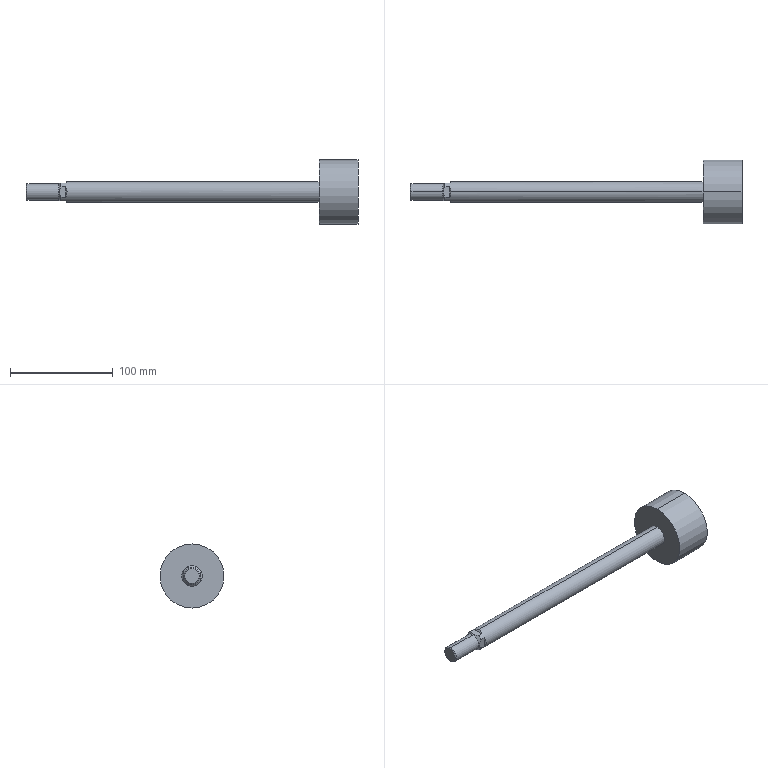Part | SolidWorks | features BaseBody 1 | 1 solid | 21 faces | box 323.5 x 62.5 x 62.5 mm | volume 202274 mm3 | plane 11 | cylinder 6 | cone 4 | commonest cylinder face diameters 16 x2 20 x2 62.5 x2
STEP:
#1=CARTESIAN_POINT('',(216.5,0.,10.));
#2=VERTEX_POINT('',#1);
#3=CARTESIAN_POINT('',(216.5,0.,-10.));
#4=VERTEX_POINT('',#3);
#5=CARTESIAN_POINT('',(216.5,0.,0.));
#6=DIRECTION('',(-1.,0.,0.));
#7=DIRECTION('',(0.,0.,1.));
#8=AXIS2_PLACEMENT_3D('',#5,#6,#7);
#9=CIRCLE('',#8,10.);
#10=EDGE_CURVE('',#2,#4,#9,.T.);
#11=ORIENTED_EDGE('',*,*,#10,.T.);
#12=CARTESIAN_POINT('',(-29.,0.,-10.));
#13=VERTEX_POINT('',#12);
#14=CARTESIAN_POINT('',(254.5,0.,-10.));
#15=DIRECTION('',(-1.,0.,0.));
#16=VECTOR('',#15,1000.);
#17=LINE('',#14,#16);
#18=EDGE_CURVE('',#4,#13,#17,.T.);
#19=ORIENTED_EDGE('',*,*,#18,.T.);
#20=CARTESIAN_POINT('',(-30.5,5.268,-8.5));
#21=VERTEX_POINT('',#20);
#22=CARTESIAN_POINT('',(-29.,0.,-10.));
#23=CARTESIAN_POINT('',(-29.,1.873,-10.));
#24=CARTESIAN_POINT('',(-29.513,3.675,-9.487));
#25=CARTESIAN_POINT('',(-30.5,5.268,-8.5));
#26=(BOUNDED_CURVE()B_SPLINE_CURVE(3,(#22,#23,#24,#25),.UNSPECIFIED.,.F.,.T.)B_SPLINE_CURVE_WITH_KNOTS((4,4),(3.142,3.696),.UNSPECIFIED.)CURVE()GEOMETRIC_REPRESENTATION_ITEM()RATIONAL_B_SPLINE_CURVE((1.,0.9745,0.9745,1.))REPRESENTATION_ITEM(''));
#27=EDGE_CURVE('',#13,#21,#26,.T.);
#28=ORIENTED_EDGE('',*,*,#27,.T.);
#29=CARTESIAN_POINT('',(-35.,5.268,-8.5));
#30=VERTEX_POINT('',#29);
#31=CARTESIAN_POINT('',(254.5,5.268,-8.5));
#32=DIRECTION('',(-1.,0.,0.));
#33=VECTOR('',#32,1000.);
#34=LINE('',#31,#33);
#35=EDGE_CURVE('',#21,#30,#34,.T.);
#36=ORIENTED_EDGE('',*,*,#35,.T.);
#37=CARTESIAN_POINT('',(-35.,8.5,-5.268));
#38=VERTEX_POINT('',#37);
#39=CARTESIAN_POINT('',(-35.,0.,0.));
#40=DIRECTION('',(1.,0.,0.));
#41=DIRECTION('',(0.,0.,1.));
#42=AXIS2_PLACEMENT_3D('',#39,#40,#41);
#43=CIRCLE('',#42,10.);
#44=EDGE_CURVE('',#30,#38,#43,.T.);
#45=ORIENTED_EDGE('',*,*,#44,.T.);
#46=CARTESIAN_POINT('',(-30.5,8.5,-5.268));
#47=VERTEX_POINT('',#46);
#48=CARTESIAN_POINT('',(254.5,8.5,-5.268));
#49=DIRECTION('',(1.,0.,0.));
#50=VECTOR('',#49,1000.);
#51=LINE('',#48,#50);
#52=EDGE_CURVE('',#38,#47,#51,.T.);
#53=ORIENTED_EDGE('',*,*,#52,.T.);
#54=CARTESIAN_POINT('',(-30.5,8.5,5.268));
#55=VERTEX_POINT('',#54);
#56=CARTESIAN_POINT('',(-30.5,8.5,-5.268));
#57=CARTESIAN_POINT('',(-28.444,10.556,-1.951));
#58=CARTESIAN_POINT('',(-28.444,10.556,1.951));
#59=CARTESIAN_POINT('',(-30.5,8.5,5.268));
#60=(BOUNDED_CURVE()B_SPLINE_CURVE(3,(#56,#57,#58,#59),.UNSPECIFIED.,.F.,.T.)B_SPLINE_CURVE_WITH_KNOTS((4,4),(2.587,3.696),.UNSPECIFIED.)CURVE()GEOMETRIC_REPRESENTATION_ITEM()RATIONAL_B_SPLINE_CURVE((1.,0.9,0.9,1.))REPRESENTATION_ITEM(''));
#61=EDGE_CURVE('',#47,#55,#60,.T.);
#62=ORIENTED_EDGE('',*,*,#61,.T.);
#63=CARTESIAN_POINT('',(-35.,8.5,5.268));
#64=VERTEX_POINT('',#63);
#65=CARTESIAN_POINT('',(254.5,8.5,5.268));
#66=DIRECTION('',(-1.,0.,0.));
#67=VECTOR('',#66,1000.);
#68=LINE('',#65,#67);
#69=EDGE_CURVE('',#55,#64,#68,.T.);
#70=ORIENTED_EDGE('',*,*,#69,.T.);
#71=CARTESIAN_POINT('',(-35.,5.268,8.5));
#72=VERTEX_POINT('',#71);
#73=CARTESIAN_POINT('',(-35.,0.,0.));
#74=DIRECTION('',(1.,0.,0.));
#75=DIRECTION('',(0.,0.,1.));
#76=AXIS2_PLACEMENT_3D('',#73,#74,#75);
#77=CIRCLE('',#76,10.);
#78=EDGE_CURVE('',#64,#72,#77,.T.);
#79=ORIENTED_EDGE('',*,*,#78,.T.);
#80=CARTESIAN_POINT('',(-30.5,5.268,8.5));
#81=VERTEX_POINT('',#80);
#82=CARTESIAN_POINT('',(254.5,5.268,8.5));
#83=DIRECTION('',(1.,0.,0.));
#84=VECTOR('',#83,1000.);
#85=LINE('',#82,#84);
#86=EDGE_CURVE('',#72,#81,#85,.T.);
#87=ORIENTED_EDGE('',*,*,#86,.T.);
#88=CARTESIAN_POINT('',(-29.,0.,10.));
#89=VERTEX_POINT('',#88);
#90=CARTESIAN_POINT('',(-30.5,5.268,8.5));
#91=CARTESIAN_POINT('',(-29.513,3.675,9.487));
#92=CARTESIAN_POINT('',(-29.,1.873,10.));
#93=CARTESIAN_POINT('',(-29.,0.,10.));
#94=(BOUNDED_CURVE()B_SPLINE_CURVE(3,(#90,#91,#92,#93),.UNSPECIFIED.,.F.,.F.)B_SPLINE_CURVE_WITH_KNOTS((4,4),(2.587,3.142),.UNSPECIFIED.)CURVE()GEOMETRIC_REPRESENTATION_ITEM()RATIONAL_B_SPLINE_CURVE((1.,0.9745,0.9745,1.))REPRESENTATION_ITEM(''));
#95=EDGE_CURVE('',#81,#89,#94,.T.);
#96=ORIENTED_EDGE('',*,*,#95,.T.);
#97=CARTESIAN_POINT('',(254.5,0.,10.));
#98=DIRECTION('',(-1.,0.,0.));
#99=VECTOR('',#98,1000.);
#100=LINE('',#97,#99);
#101=EDGE_CURVE('',#2,#89,#100,.T.);
#102=ORIENTED_EDGE('',*,*,#101,.F.);
#103=EDGE_LOOP('',(#11,#19,#28,#36,#45,#53,#62,#70,#79,#87,#96,#102));
#104=FACE_OUTER_BOUND('',#103,.T.);
#105=CARTESIAN_POINT('',(254.5,0.,0.));
#106=DIRECTION('',(-1.,0.,0.));
#107=DIRECTION('',(0.,0.,1.));
#108=AXIS2_PLACEMENT_3D('',#105,#106,#107);
#109=CYLINDRICAL_SURFACE('',#108,10.);
#110=ADVANCED_FACE('',(#104),#109,.T.);
#111=CARTESIAN_POINT('',(-37.,0.,-8.));
#112=VERTEX_POINT('',#111);
#113=CARTESIAN_POINT('',(-37.,0.,8.));
#114=VERTEX_POINT('',#113);
#115=CARTESIAN_POINT('',(-37.,0.,0.));
#116=DIRECTION('',(1.,0.,0.));
#117=DIRECTION('',(0.,0.,-1.));
#118=AXIS2_PLACEMENT_3D('',#115,#116,#117);
#119=CIRCLE('',#118,8.);
#120=EDGE_CURVE('',#112,#114,#119,.T.);
#121=ORIENTED_EDGE('',*,*,#120,.T.);
#122=CARTESIAN_POINT('',(-36.5,0.,8.5));
#123=VERTEX_POINT('',#122);
#124=CARTESIAN_POINT('',(-35.,0.,10.));
#125=DIRECTION('',(0.7071,0.,0.7071));
#126=VECTOR('',#125,1000.);
#127=LINE('',#124,#126);
#128=EDGE_CURVE('',#114,#123,#127,.T.);
#129=ORIENTED_EDGE('',*,*,#128,.T.);
#130=CARTESIAN_POINT('',(-35.,5.268,8.5));
#131=CARTESIAN_POINT('',(-35.432,4.448,8.5));
#132=CARTESIAN_POINT('',(-35.804,3.607,8.5));
#133=CARTESIAN_POINT('',(-36.207,2.288,8.5));
#134=CARTESIAN_POINT('',(-36.316,1.837,8.5));
#135=CARTESIAN_POINT('',(-36.463,0.9184,8.5));
#136=CARTESIAN_POINT('',(-36.5,0.4592,8.5));
#137=CARTESIAN_POINT('',(-36.5,0.,8.5));
#138=B_SPLINE_CURVE_WITH_KNOTS('',3,(#130,#131,#132,#133,#134,#135,#136,#137),.UNSPECIFIED.,.F.,.F.,(4,2,2,4),(0.,0.002754,0.004131,0.005508),.UNSPECIFIED.);
#139=EDGE_CURVE('',#72,#123,#138,.T.);
#140=ORIENTED_EDGE('',*,*,#139,.F.);
#141=ORIENTED_EDGE('',*,*,#78,.F.);
#142=CARTESIAN_POINT('',(-35.,8.5,5.268));
#143=CARTESIAN_POINT('',(-35.432,8.5,4.448));
#144=CARTESIAN_POINT('',(-35.804,8.5,3.607));
#145=CARTESIAN_POINT('',(-36.207,8.5,2.289));
#146=CARTESIAN_POINT('',(-36.315,8.5,1.838));
#147=CARTESIAN_POINT('',(-36.462,8.5,0.919));
#148=CARTESIAN_POINT('',(-36.5,8.5,0.4598));
#149=CARTESIAN_POINT('',(-36.5,8.5,-0.4584));
#150=CARTESIAN_POINT('',(-36.463,8.5,-0.9173));
#151=CARTESIAN_POINT('',(-36.316,8.5,-1.835));
#152=CARTESIAN_POINT('',(-36.208,8.5,-2.287));
#153=CARTESIAN_POINT('',(-35.805,8.5,-3.606));
#154=CARTESIAN_POINT('',(-35.432,8.5,-4.448));
#155=CARTESIAN_POINT('',(-35.,8.5,-5.268));
#156=B_SPLINE_CURVE_WITH_KNOTS('',3,(#142,#143,#144,#145,#146,#147,#148,#149,#150,#151,#152,#153,#154,#155),.UNSPECIFIED.,.F.,.F.,(4,2,2,2,2,2,4),(0.,0.002753,0.00413,0.005507,0.006884,0.00826,0.01101),.UNSPECIFIED.);
#157=EDGE_CURVE('',#64,#38,#156,.T.);
#158=ORIENTED_EDGE('',*,*,#157,.T.);
#159=ORIENTED_EDGE('',*,*,#44,.F.);
#160=CARTESIAN_POINT('',(-36.5,0.,-8.5));
#161=VERTEX_POINT('',#160);
#162=CARTESIAN_POINT('',(-35.,5.268,-8.5));
#163=CARTESIAN_POINT('',(-35.432,4.448,-8.5));
#164=CARTESIAN_POINT('',(-35.804,3.607,-8.5));
#165=CARTESIAN_POINT('',(-36.207,2.288,-8.5));
#166=CARTESIAN_POINT('',(-36.316,1.837,-8.5));
#167=CARTESIAN_POINT('',(-36.463,0.9184,-8.5));
#168=CARTESIAN_POINT('',(-36.5,0.4592,-8.5));
#169=CARTESIAN_POINT('',(-36.5,0.,-8.5));
#170=B_SPLINE_CURVE_WITH_KNOTS('',3,(#162,#163,#164,#165,#166,#167,#168,#169),.UNSPECIFIED.,.F.,.F.,(4,2,2,4),(0.,0.002754,0.004131,0.005508),.UNSPECIFIED.);
#171=EDGE_CURVE('',#30,#161,#170,.T.);
#172=ORIENTED_EDGE('',*,*,#171,.T.);
#173=CARTESIAN_POINT('',(-35.,0.,-10.));
#174=DIRECTION('',(0.7071,0.,-0.7071));
#175=VECTOR('',#174,1000.);
#176=LINE('',#173,#175);
#177=EDGE_CURVE('',#112,#161,#176,.T.);
#178=ORIENTED_EDGE('',*,*,#177,.F.);
#179=EDGE_LOOP('',(#121,#129,#140,#141,#158,#159,#172,#178));
#180=FACE_OUTER_BOUND('',#179,.T.);
#181=CARTESIAN_POINT('',(-35.,0.,0.));
#182=DIRECTION('',(1.,0.,0.));
#183=DIRECTION('',(0.,0.,-1.));
#184=AXIS2_PLACEMENT_3D('',#181,#182,#183);
#185=CONICAL_SURFACE('',#184,10.,0.7854);
#186=ADVANCED_FACE('',(#180),#185,.T.);
#187=ORIENTED_EDGE('',*,*,#120,.F.);
#188=CARTESIAN_POINT('',(-68.08,0.,-8.));
#189=VERTEX_POINT('',#188);
#190=CARTESIAN_POINT('',(254.5,0.,-8.));
#191=DIRECTION('',(-1.,0.,0.));
#192=VECTOR('',#191,1000.);
#193=LINE('',#190,#192);
#194=EDGE_CURVE('',#112,#189,#193,.T.);
#195=ORIENTED_EDGE('',*,*,#194,.T.);
#196=CARTESIAN_POINT('',(-68.08,0.,8.));
#197=VERTEX_POINT('',#196);
#198=CARTESIAN_POINT('',(-68.08,0.,0.));
#199=DIRECTION('',(1.,0.,0.));
#200=DIRECTION('',(0.,0.,1.));
#201=AXIS2_PLACEMENT_3D('',#198,#199,#200);
#202=CIRCLE('',#201,8.);
#203=EDGE_CURVE('',#189,#197,#202,.T.);
#204=ORIENTED_EDGE('',*,*,#203,.T.);
#205=CARTESIAN_POINT('',(254.5,0.,8.));
#206=DIRECTION('',(-1.,0.,0.));
#207=VECTOR('',#206,1000.);
#208=LINE('',#205,#207);
#209=EDGE_CURVE('',#114,#197,#208,.T.);
#210=ORIENTED_EDGE('',*,*,#209,.F.);
#211=EDGE_LOOP('',(#187,#195,#204,#210));
#212=FACE_OUTER_BOUND('',#211,.T.);
#213=CARTESIAN_POINT('',(254.5,0.,0.));
#214=DIRECTION('',(-1.,0.,0.));
#215=DIRECTION('',(0.,0.,1.));
#216=AXIS2_PLACEMENT_3D('',#213,#214,#215);
#217=CYLINDRICAL_SURFACE('',#216,8.);
#218=ADVANCED_FACE('',(#212),#217,.T.);
#219=CARTESIAN_POINT('',(254.5,0.,31.25));
#220=VERTEX_POINT('',#219);
#221=CARTESIAN_POINT('',(254.5,0.,-31.25));
#222=VERTEX_POINT('',#221);
#223=CARTESIAN_POINT('',(254.5,0.,0.));
#224=DIRECTION('',(-1.,0.,0.));
#225=DIRECTION('',(0.,0.,1.));
#226=AXIS2_PLACEMENT_3D('',#223,#224,#225);
#227=CIRCLE('',#226,31.25);
#228=EDGE_CURVE('',#220,#222,#227,.T.);
#229=ORIENTED_EDGE('',*,*,#228,.T.);
#230=CARTESIAN_POINT('',(216.5,0.,-31.25));
#231=VERTEX_POINT('',#230);
#232=CARTESIAN_POINT('',(254.5,0.,-31.25));
#233=DIRECTION('',(-1.,0.,0.));
#234=VECTOR('',#233,1000.);
#235=LINE('',#232,#234);
#236=EDGE_CURVE('',#222,#231,#235,.T.);
#237=ORIENTED_EDGE('',*,*,#236,.T.);
#238=CARTESIAN_POINT('',(216.5,0.,31.25));
#239=VERTEX_POINT('',#238);
#240=CARTESIAN_POINT('',(216.5,0.,0.));
#241=DIRECTION('',(1.,0.,0.));
#242=DIRECTION('',(0.,0.,1.));
#243=AXIS2_PLACEMENT_3D('',#240,#241,#242);
#244=CIRCLE('',#243,31.25);
#245=EDGE_CURVE('',#231,#239,#244,.T.);
#246=ORIENTED_EDGE('',*,*,#245,.T.);
#247=CARTESIAN_POINT('',(254.5,0.,31.25));
#248=DIRECTION('',(-1.,0.,0.));
#249=VECTOR('',#248,1000.);
#250=LINE('',#247,#249);
#251=EDGE_CURVE('',#220,#239,#250,.T.);
#252=ORIENTED_EDGE('',*,*,#251,.F.);
#253=EDGE_LOOP('',(#229,#237,#246,#252));
#254=FACE_OUTER_BOUND('',#253,.T.);
#255=CARTESIAN_POINT('',(254.5,0.,0.));
#256=DIRECTION('',(-1.,0.,0.));
#257=DIRECTION('',(0.,0.,1.));
#258=AXIS2_PLACEMENT_3D('',#255,#256,#257);
#259=CYLINDRICAL_SURFACE('',#258,31.25);
#260=ADVANCED_FACE('',(#254),#259,.T.);
#261=CARTESIAN_POINT('',(-69.,0.,-7.08));
#262=VERTEX_POINT('',#261);
#263=CARTESIAN_POINT('',(-69.,0.,7.08));
#264=VERTEX_POINT('',#263);
#265=CARTESIAN_POINT('',(-69.,0.,0.));
#266=DIRECTION('',(1.,0.,0.));
#267=DIRECTION('',(0.,0.,-1.));
#268=AXIS2_PLACEMENT_3D('',#265,#266,#267);
#269=CIRCLE('',#268,7.08);
#270=EDGE_CURVE('',#262,#264,#269,.T.);
#271=ORIENTED_EDGE('',*,*,#270,.T.);
#272=CARTESIAN_POINT('',(-68.08,0.,8.));
#273=DIRECTION('',(0.7071,0.,0.7071));
#274=VECTOR('',#273,1000.);
#275=LINE('',#272,#274);
#276=EDGE_CURVE('',#264,#197,#275,.T.);
#277=ORIENTED_EDGE('',*,*,#276,.T.);
#278=ORIENTED_EDGE('',*,*,#203,.F.);
#279=CARTESIAN_POINT('',(-68.08,0.,-8.));
#280=DIRECTION('',(0.7071,0.,-0.7071));
#281=VECTOR('',#280,1000.);
#282=LINE('',#279,#281);
#283=EDGE_CURVE('',#262,#189,#282,.T.);
#284=ORIENTED_EDGE('',*,*,#283,.F.);
#285=EDGE_LOOP('',(#271,#277,#278,#284));
#286=FACE_OUTER_BOUND('',#285,.T.);
#287=CARTESIAN_POINT('',(-68.08,0.,0.));
#288=DIRECTION('',(1.,0.,0.));
#289=DIRECTION('',(0.,0.,-1.));
#290=AXIS2_PLACEMENT_3D('',#287,#288,#289);
#291=CONICAL_SURFACE('',#290,8.,0.7854);
#292=ADVANCED_FACE('',(#286),#291,.T.);
#293=ORIENTED_EDGE('',*,*,#18,.F.);
#294=CARTESIAN_POINT('',(216.5,0.,0.));
#295=DIRECTION('',(-1.,0.,0.));
#296=DIRECTION('',(0.,0.,1.));
#297=AXIS2_PLACEMENT_3D('',#294,#295,#296);
#298=CIRCLE('',#297,10.);
#299=EDGE_CURVE('',#4,#2,#298,.T.);
#300=ORIENTED_EDGE('',*,*,#299,.T.);
#301=ORIENTED_EDGE('',*,*,#101,.T.);
#302=CARTESIAN_POINT('',(-30.5,-5.268,8.5));
#303=VERTEX_POINT('',#302);
#304=CARTESIAN_POINT('',(-29.,0.,10.));
#305=CARTESIAN_POINT('',(-29.,-1.873,10.));
#306=CARTESIAN_POINT('',(-29.513,-3.675,9.487));
#307=CARTESIAN_POINT('',(-30.5,-5.268,8.5));
#308=(BOUNDED_CURVE()B_SPLINE_CURVE(3,(#304,#305,#306,#307),.UNSPECIFIED.,.F.,.F.)B_SPLINE_CURVE_WITH_KNOTS((4,4),(3.142,3.696),.UNSPECIFIED.)CURVE()GEOMETRIC_REPRESENTATION_ITEM()RATIONAL_B_SPLINE_CURVE((1.,0.9745,0.9745,1.))REPRESENTATION_ITEM(''));
#309=EDGE_CURVE('',#89,#303,#308,.T.);
#310=ORIENTED_EDGE('',*,*,#309,.T.);
#311=CARTESIAN_POINT('',(-35.,-5.268,8.5));
#312=VERTEX_POINT('',#311);
#313=CARTESIAN_POINT('',(254.5,-5.268,8.5));
#314=DIRECTION('',(-1.,0.,0.));
#315=VECTOR('',#314,1000.);
#316=LINE('',#313,#315);
#317=EDGE_CURVE('',#303,#312,#316,.T.);
#318=ORIENTED_EDGE('',*,*,#317,.T.);
#319=CARTESIAN_POINT('',(-35.,-8.5,5.268));
#320=VERTEX_POINT('',#319);
#321=CARTESIAN_POINT('',(-35.,0.,0.));
#322=DIRECTION('',(1.,0.,0.));
#323=DIRECTION('',(0.,0.,1.));
#324=AXIS2_PLACEMENT_3D('',#321,#322,#323);
#325=CIRCLE('',#324,10.);
#326=EDGE_CURVE('',#312,#320,#325,.T.);
#327=ORIENTED_EDGE('',*,*,#326,.T.);
#328=CARTESIAN_POINT('',(-30.5,-8.5,5.268));
#329=VERTEX_POINT('',#328);
#330=CARTESIAN_POINT('',(254.5,-8.5,5.268));
#331=DIRECTION('',(1.,0.,0.));
#332=VECTOR('',#331,1000.);
#333=LINE('',#330,#332);
#334=EDGE_CURVE('',#320,#329,#333,.T.);
#335=ORIENTED_EDGE('',*,*,#334,.T.);
#336=CARTESIAN_POINT('',(-30.5,-8.5,-5.268));
#337=VERTEX_POINT('',#336);
#338=CARTESIAN_POINT('',(-30.5,-8.5,5.268));
#339=CARTESIAN_POINT('',(-28.444,-10.556,1.951));
#340=CARTESIAN_POINT('',(-28.444,-10.556,-1.951));
#341=CARTESIAN_POINT('',(-30.5,-8.5,-5.268));
#342=(BOUNDED_CURVE()B_SPLINE_CURVE(3,(#338,#339,#340,#341),.UNSPECIFIED.,.F.,.F.)B_SPLINE_CURVE_WITH_KNOTS((4,4),(2.587,3.696),.UNSPECIFIED.)CURVE()GEOMETRIC_REPRESENTATION_ITEM()RATIONAL_B_SPLINE_CURVE((1.,0.9,0.9,1.))REPRESENTATION_ITEM(''));
#343=EDGE_CURVE('',#329,#337,#342,.T.);
#344=ORIENTED_EDGE('',*,*,#343,.T.);
#345=CARTESIAN_POINT('',(-35.,-8.5,-5.268));
#346=VERTEX_POINT('',#345);
#347=CARTESIAN_POINT('',(254.5,-8.5,-5.268));
#348=DIRECTION('',(-1.,0.,0.));
#349=VECTOR('',#348,1000.);
#350=LINE('',#347,#349);
#351=EDGE_CURVE('',#337,#346,#350,.T.);
#352=ORIENTED_EDGE('',*,*,#351,.T.);
#353=CARTESIAN_POINT('',(-35.,-5.268,-8.5));
#354=VERTEX_POINT('',#353);
#355=CARTESIAN_POINT('',(-35.,0.,0.));
#356=DIRECTION('',(1.,0.,0.));
#357=DIRECTION('',(0.,0.,1.));
#358=AXIS2_PLACEMENT_3D('',#355,#356,#357);
#359=CIRCLE('',#358,10.);
#360=EDGE_CURVE('',#346,#354,#359,.T.);
#361=ORIENTED_EDGE('',*,*,#360,.T.);
#362=CARTESIAN_POINT('',(-30.5,-5.268,-8.5));
#363=VERTEX_POINT('',#362);
#364=CARTESIAN_POINT('',(254.5,-5.268,-8.5));
#365=DIRECTION('',(1.,0.,0.));
#366=VECTOR('',#365,1000.);
#367=LINE('',#364,#366);
#368=EDGE_CURVE('',#354,#363,#367,.T.);
#369=ORIENTED_EDGE('',*,*,#368,.T.);
#370=CARTESIAN_POINT('',(-30.5,-5.268,-8.5));
#371=CARTESIAN_POINT('',(-29.513,-3.675,-9.487));
#372=CARTESIAN_POINT('',(-29.,-1.873,-10.));
#373=CARTESIAN_POINT('',(-29.,0.,-10.));
#374=(BOUNDED_CURVE()B_SPLINE_CURVE(3,(#370,#371,#372,#373),.UNSPECIFIED.,.F.,.T.)B_SPLINE_CURVE_WITH_KNOTS((4,4),(2.587,3.142),.UNSPECIFIED.)CURVE()GEOMETRIC_REPRESENTATION_ITEM()RATIONAL_B_SPLINE_CURVE((1.,0.9745,0.9745,1.))REPRESENTATION_ITEM(''));
#375=EDGE_CURVE('',#363,#13,#374,.T.);
#376=ORIENTED_EDGE('',*,*,#375,.T.);
#377=EDGE_LOOP('',(#293,#300,#301,#310,#318,#327,#335,#344,#352,#361,#369,#376));
#378=FACE_OUTER_BOUND('',#377,.T.);
#379=CARTESIAN_POINT('',(254.5,0.,0.));
#380=DIRECTION('',(-1.,0.,0.));
#381=DIRECTION('',(0.,0.,1.));
#382=AXIS2_PLACEMENT_3D('',#379,#380,#381);
#383=CYLINDRICAL_SURFACE('',#382,10.);
#384=ADVANCED_FACE('',(#378),#383,.T.);
#385=ORIENTED_EDGE('',*,*,#95,.F.);
#386=CARTESIAN_POINT('',(-30.5,8.5,8.5));
#387=DIRECTION('',(0.,-1.,0.));
#388=VECTOR('',#387,1000.);
#389=LINE('',#386,#388);
#390=EDGE_CURVE('',#81,#303,#389,.T.);
#391=ORIENTED_EDGE('',*,*,#390,.T.);
#392=ORIENTED_EDGE('',*,*,#309,.F.);
#393=EDGE_LOOP('',(#385,#391,#392));
#394=FACE_OUTER_BOUND('',#393,.T.);
#395=CARTESIAN_POINT('',(-29.,8.5,10.));
#396=DIRECTION('',(-0.7071,0.,0.7071));
#397=DIRECTION('',(0.7071,0.,0.7071));
#398=AXIS2_PLACEMENT_3D('',#395,#396,#397);
#399=PLANE('',#398);
#400=ADVANCED_FACE('',(#394),#399,.T.);
#401=ORIENTED_EDGE('',*,*,#86,.F.);
#402=ORIENTED_EDGE('',*,*,#139,.T.);
#403=CARTESIAN_POINT('',(-36.5,0.,8.5));
#404=CARTESIAN_POINT('',(-36.5,-0.459,8.5));
#405=CARTESIAN_POINT('',(-36.463,-0.9179,8.5));
#406=CARTESIAN_POINT('',(-36.316,-1.835,8.5));
#407=CARTESIAN_POINT('',(-36.208,-2.287,8.5));
#408=CARTESIAN_POINT('',(-35.805,-3.607,8.5));
#409=CARTESIAN_POINT('',(-35.432,-4.448,8.5));
#410=CARTESIAN_POINT('',(-35.,-5.268,8.5));
#411=B_SPLINE_CURVE_WITH_KNOTS('',3,(#403,#404,#405,#406,#407,#408,#409,#410),.UNSPECIFIED.,.F.,.F.,(4,2,2,4),(0.005508,0.006884,0.008261,0.01101),.UNSPECIFIED.);
#412=EDGE_CURVE('',#123,#312,#411,.T.);
#413=ORIENTED_EDGE('',*,*,#412,.T.);
#414=ORIENTED_EDGE('',*,*,#317,.F.);
#415=ORIENTED_EDGE('',*,*,#390,.F.);
#416=EDGE_LOOP('',(#401,#402,#413,#414,#415));
#417=FACE_OUTER_BOUND('',#416,.T.);
#418=CARTESIAN_POINT('',(-30.5,8.5,8.5));
#419=DIRECTION('',(0.,0.,1.));
#420=DIRECTION('',(1.,0.,0.));
#421=AXIS2_PLACEMENT_3D('',#418,#419,#420);
#422=PLANE('',#421);
#423=ADVANCED_FACE('',(#417),#422,.T.);
#424=ORIENTED_EDGE('',*,*,#128,.F.);
#425=CARTESIAN_POINT('',(-37.,0.,0.));
#426=DIRECTION('',(1.,0.,0.));
#427=DIRECTION('',(0.,0.,-1.));
#428=AXIS2_PLACEMENT_3D('',#425,#426,#427);
#429=CIRCLE('',#428,8.);
#430=EDGE_CURVE('',#114,#112,#429,.T.);
#431=ORIENTED_EDGE('',*,*,#430,.T.);
#432=ORIENTED_EDGE('',*,*,#177,.T.);
#433=CARTESIAN_POINT('',(-36.5,0.,-8.5));
#434=CARTESIAN_POINT('',(-36.5,-0.459,-8.5));
#435=CARTESIAN_POINT('',(-36.463,-0.9179,-8.5));
#436=CARTESIAN_POINT('',(-36.316,-1.835,-8.5));
#437=CARTESIAN_POINT('',(-36.208,-2.287,-8.5));
#438=CARTESIAN_POINT('',(-35.805,-3.607,-8.5));
#439=CARTESIAN_POINT('',(-35.432,-4.448,-8.5));
#440=CARTESIAN_POINT('',(-35.,-5.268,-8.5));
#441=B_SPLINE_CURVE_WITH_KNOTS('',3,(#433,#434,#435,#436,#437,#438,#439,#440),.UNSPECIFIED.,.F.,.F.,(4,2,2,4),(0.005508,0.006884,0.008261,0.01101),.UNSPECIFIED.);
#442=EDGE_CURVE('',#161,#354,#441,.T.);
#443=ORIENTED_EDGE('',*,*,#442,.T.);
#444=ORIENTED_EDGE('',*,*,#360,.F.);
#445=CARTESIAN_POINT('',(-35.,-8.5,-5.268));
#446=CARTESIAN_POINT('',(-35.432,-8.5,-4.448));
#447=CARTESIAN_POINT('',(-35.804,-8.5,-3.607));
#448=CARTESIAN_POINT('',(-36.207,-8.5,-2.289));
#449=CARTESIAN_POINT('',(-36.315,-8.5,-1.838));
#450=CARTESIAN_POINT('',(-36.462,-8.5,-0.919));
#451=CARTESIAN_POINT('',(-36.5,-8.5,-0.4598));
#452=CARTESIAN_POINT('',(-36.5,-8.5,0.4584));
#453=CARTESIAN_POINT('',(-36.463,-8.5,0.9173));
#454=CARTESIAN_POINT('',(-36.316,-8.5,1.835));
#455=CARTESIAN_POINT('',(-36.208,-8.5,2.287));
#456=CARTESIAN_POINT('',(-35.805,-8.5,3.606));
#457=CARTESIAN_POINT('',(-35.432,-8.5,4.448));
#458=CARTESIAN_POINT('',(-35.,-8.5,5.268));
#459=B_SPLINE_CURVE_WITH_KNOTS('',3,(#445,#446,#447,#448,#449,#450,#451,#452,#453,#454,#455,#456,#457,#458),.UNSPECIFIED.,.F.,.F.,(4,2,2,2,2,2,4),(0.,0.002753,0.00413,0.005507,0.006884,0.00826,0.01101),.UNSPECIFIED.);
#460=EDGE_CURVE('',#346,#320,#459,.T.);
#461=ORIENTED_EDGE('',*,*,#460,.T.);
#462=ORIENTED_EDGE('',*,*,#326,.F.);
#463=ORIENTED_EDGE('',*,*,#412,.F.);
#464=EDGE_LOOP('',(#424,#431,#432,#443,#444,#461,#462,#463));
#465=FACE_OUTER_BOUND('',#464,.T.);
#466=CARTESIAN_POINT('',(-35.,0.,0.));
#467=DIRECTION('',(1.,0.,0.));
#468=DIRECTION('',(0.,0.,-1.));
#469=AXIS2_PLACEMENT_3D('',#466,#467,#468);
#470=CONICAL_SURFACE('',#469,10.,0.7854);
#471=ADVANCED_FACE('',(#465),#470,.T.);
#472=ORIENTED_EDGE('',*,*,#52,.F.);
#473=ORIENTED_EDGE('',*,*,#157,.F.);
#474=ORIENTED_EDGE('',*,*,#69,.F.);
#475=CARTESIAN_POINT('',(-30.5,8.5,8.5));
#476=DIRECTION('',(0.,0.,-1.));
#477=VECTOR('',#476,1000.);
#478=LINE('',#475,#477);
#479=EDGE_CURVE('',#55,#47,#478,.T.);
#480=ORIENTED_EDGE('',*,*,#479,.T.);
#481=EDGE_LOOP('',(#472,#473,#474,#480));
#482=FACE_OUTER_BOUND('',#481,.T.);
#483=CARTESIAN_POINT('',(-71.7,8.5,8.5));
#484=DIRECTION('',(0.,1.,0.));
#485=DIRECTION('',(0.,0.,1.));
#486=AXIS2_PLACEMENT_3D('',#483,#484,#485);
#487=PLANE('',#486);
#488=ADVANCED_FACE('',(#482),#487,.T.);
#489=ORIENTED_EDGE('',*,*,#61,.F.);
#490=ORIENTED_EDGE('',*,*,#479,.F.);
#491=EDGE_LOOP('',(#489,#490));
#492=FACE_OUTER_BOUND('',#491,.T.);
#493=CARTESIAN_POINT('',(-30.5,8.5,8.5));
#494=DIRECTION('',(-0.7071,0.7071,0.));
#495=DIRECTION('',(-0.7071,-0.7071,0.));
#496=AXIS2_PLACEMENT_3D('',#493,#494,#495);
#497=PLANE('',#496);
#498=ADVANCED_FACE('',(#492),#497,.T.);
#499=ORIENTED_EDGE('',*,*,#368,.F.);
#500=ORIENTED_EDGE('',*,*,#442,.F.);
#501=ORIENTED_EDGE('',*,*,#171,.F.);
#502=ORIENTED_EDGE('',*,*,#35,.F.);
#503=CARTESIAN_POINT('',(-30.5,8.5,-8.5));
#504=DIRECTION('',(0.,-1.,0.));
#505=VECTOR('',#504,1000.);
#506=LINE('',#503,#505);
#507=EDGE_CURVE('',#21,#363,#506,.T.);
#508=ORIENTED_EDGE('',*,*,#507,.T.);
#509=EDGE_LOOP('',(#499,#500,#501,#502,#508));
#510=FACE_OUTER_BOUND('',#509,.T.);
#511=CARTESIAN_POINT('',(-71.7,8.5,-8.5));
#512=DIRECTION('',(0.,0.,-1.));
#513=DIRECTION('',(-1.,0.,0.));
#514=AXIS2_PLACEMENT_3D('',#511,#512,#513);
#515=PLANE('',#514);
#516=ADVANCED_FACE('',(#510),#515,.T.);
#517=ORIENTED_EDGE('',*,*,#375,.F.);
#518=ORIENTED_EDGE('',*,*,#507,.F.);
#519=ORIENTED_EDGE('',*,*,#27,.F.);
#520=EDGE_LOOP('',(#517,#518,#519));
#521=FACE_OUTER_BOUND('',#520,.T.);
#522=CARTESIAN_POINT('',(-30.5,8.5,-8.5));
#523=DIRECTION('',(-0.7071,0.,-0.7071));
#524=DIRECTION('',(-0.7071,0.,0.7071));
#525=AXIS2_PLACEMENT_3D('',#522,#523,#524);
#526=PLANE('',#525);
#527=ADVANCED_FACE('',(#521),#526,.T.);
#528=ORIENTED_EDGE('',*,*,#334,.F.);
#529=ORIENTED_EDGE('',*,*,#460,.F.);
#530=ORIENTED_EDGE('',*,*,#351,.F.);
#531=CARTESIAN_POINT('',(-30.5,-8.5,8.5));
#532=DIRECTION('',(0.,0.,1.));
#533=VECTOR('',#532,1000.);
#534=LINE('',#531,#533);
#535=EDGE_CURVE('',#337,#329,#534,.T.);
#536=ORIENTED_EDGE('',*,*,#535,.T.);
#537=EDGE_LOOP('',(#528,#529,#530,#536));
#538=FACE_OUTER_BOUND('',#537,.T.);
#539=CARTESIAN_POINT('',(-30.5,-8.5,8.5));
#540=DIRECTION('',(0.,-1.,0.));
#541=DIRECTION('',(0.,0.,-1.));
#542=AXIS2_PLACEMENT_3D('',#539,#540,#541);
#543=PLANE('',#542);
#544=ADVANCED_FACE('',(#538),#543,.T.);
#545=ORIENTED_EDGE('',*,*,#343,.F.);
#546=ORIENTED_EDGE('',*,*,#535,.F.);
#547=EDGE_LOOP('',(#545,#546));
#548=FACE_OUTER_BOUND('',#547,.T.);
#549=CARTESIAN_POINT('',(-29.,-10.,8.5));
#550=DIRECTION('',(-0.7071,-0.7071,0.));
#551=DIRECTION('',(0.7071,-0.7071,0.));
#552=AXIS2_PLACEMENT_3D('',#549,#550,#551);
#553=PLANE('',#552);
#554=ADVANCED_FACE('',(#548),#553,.T.);
#555=ORIENTED_EDGE('',*,*,#10,.F.);
#556=ORIENTED_EDGE('',*,*,#299,.F.);
#557=EDGE_LOOP('',(#555,#556));
#558=FACE_BOUND('',#557,.T.);
#559=CARTESIAN_POINT('',(216.5,0.,0.));
#560=DIRECTION('',(1.,0.,0.));
#561=DIRECTION('',(0.,0.,1.));
#562=AXIS2_PLACEMENT_3D('',#559,#560,#561);
#563=CIRCLE('',#562,31.25);
#564=EDGE_CURVE('',#239,#231,#563,.T.);
#565=ORIENTED_EDGE('',*,*,#564,.F.);
#566=ORIENTED_EDGE('',*,*,#245,.F.);
#567=EDGE_LOOP('',(#565,#566));
#568=FACE_OUTER_BOUND('',#567,.T.);
#569=CARTESIAN_POINT('',(216.5,10.,0.));
#570=DIRECTION('',(1.,0.,0.));
#571=DIRECTION('',(0.,0.,-1.));
#572=AXIS2_PLACEMENT_3D('',#569,#570,#571);
#573=PLANE('',#572);
#574=ADVANCED_FACE('',(#558,#568),#573,.F.);
#575=ORIENTED_EDGE('',*,*,#194,.F.);
#576=ORIENTED_EDGE('',*,*,#430,.F.);
#577=ORIENTED_EDGE('',*,*,#209,.T.);
#578=CARTESIAN_POINT('',(-68.08,0.,0.));
#579=DIRECTION('',(1.,0.,0.));
#580=DIRECTION('',(0.,0.,1.));
#581=AXIS2_PLACEMENT_3D('',#578,#579,#580);
#582=CIRCLE('',#581,8.);
#583=EDGE_CURVE('',#197,#189,#582,.T.);
#584=ORIENTED_EDGE('',*,*,#583,.T.);
#585=EDGE_LOOP('',(#575,#576,#577,#584));
#586=FACE_OUTER_BOUND('',#585,.T.);
#587=CARTESIAN_POINT('',(254.5,0.,0.));
#588=DIRECTION('',(-1.,0.,0.));
#589=DIRECTION('',(0.,0.,1.));
#590=AXIS2_PLACEMENT_3D('',#587,#588,#589);
#591=CYLINDRICAL_SURFACE('',#590,8.);
#592=ADVANCED_FACE('',(#586),#591,.T.);
#593=ORIENTED_EDGE('',*,*,#236,.F.);
#594=CARTESIAN_POINT('',(254.5,0.,0.));
#595=DIRECTION('',(-1.,0.,0.));
#596=DIRECTION('',(0.,0.,1.));
#597=AXIS2_PLACEMENT_3D('',#594,#595,#596);
#598=CIRCLE('',#597,31.25);
#599=EDGE_CURVE('',#222,#220,#598,.T.);
#600=ORIENTED_EDGE('',*,*,#599,.T.);
#601=ORIENTED_EDGE('',*,*,#251,.T.);
#602=ORIENTED_EDGE('',*,*,#564,.T.);
#603=EDGE_LOOP('',(#593,#600,#601,#602));
#604=FACE_OUTER_BOUND('',#603,.T.);
#605=CARTESIAN_POINT('',(254.5,0.,0.));
#606=DIRECTION('',(-1.,0.,0.));
#607=DIRECTION('',(0.,0.,1.));
#608=AXIS2_PLACEMENT_3D('',#605,#606,#607);
#609=CYLINDRICAL_SURFACE('',#608,31.25);
#610=ADVANCED_FACE('',(#604),#609,.T.);
#611=ORIENTED_EDGE('',*,*,#276,.F.);
#612=CARTESIAN_POINT('',(-69.,0.,0.));
#613=DIRECTION('',(1.,0.,0.));
#614=DIRECTION('',(0.,0.,-1.));
#615=AXIS2_PLACEMENT_3D('',#612,#613,#614);
#616=CIRCLE('',#615,7.08);
#617=EDGE_CURVE('',#264,#262,#616,.T.);
#618=ORIENTED_EDGE('',*,*,#617,.T.);
#619=ORIENTED_EDGE('',*,*,#283,.T.);
#620=ORIENTED_EDGE('',*,*,#583,.F.);
#621=EDGE_LOOP('',(#611,#618,#619,#620));
#622=FACE_OUTER_BOUND('',#621,.T.);
#623=CARTESIAN_POINT('',(-68.08,0.,0.));
#624=DIRECTION('',(1.,0.,0.));
#625=DIRECTION('',(0.,0.,-1.));
#626=AXIS2_PLACEMENT_3D('',#623,#624,#625);
#627=CONICAL_SURFACE('',#626,8.,0.7854);
#628=ADVANCED_FACE('',(#622),#627,.T.);
#629=ORIENTED_EDGE('',*,*,#228,.F.);
#630=ORIENTED_EDGE('',*,*,#599,.F.);
#631=EDGE_LOOP('',(#629,#630));
#632=FACE_OUTER_BOUND('',#631,.T.);
#633=CARTESIAN_POINT('',(254.5,31.25,0.));
#634=DIRECTION('',(-1.,0.,0.));
#635=DIRECTION('',(0.,0.,1.));
#636=AXIS2_PLACEMENT_3D('',#633,#634,#635);
#637=PLANE('',#636);
#638=ADVANCED_FACE('',(#632),#637,.F.);
#639=ORIENTED_EDGE('',*,*,#270,.F.);
#640=ORIENTED_EDGE('',*,*,#617,.F.);
#641=EDGE_LOOP('',(#639,#640));
#642=FACE_OUTER_BOUND('',#641,.T.);
#643=CARTESIAN_POINT('',(-69.,0.,0.));
#644=DIRECTION('',(1.,0.,0.));
#645=DIRECTION('',(0.,0.,-1.));
#646=AXIS2_PLACEMENT_3D('',#643,#644,#645);
#647=PLANE('',#646);
#648=ADVANCED_FACE('',(#642),#647,.F.);
#649=CLOSED_SHELL('',(#110,#186,#218,#260,#292,#384,#400,#423,#471,#488,#498,#516,#527,#544,#554,#574,#592,#610,#628,#638,#648));
#650=MANIFOLD_SOLID_BREP('',#649);
#651=CARTESIAN_POINT('',(0.,0.,0.));
#652=DIRECTION('',(0.,0.,1.));
#653=DIRECTION('',(1.,0.,0.));
#654=AXIS2_PLACEMENT_3D('',#651,#652,#653);
#655=(LENGTH_UNIT()NAMED_UNIT(*)SI_UNIT(.MILLI.,.METRE.));
#656=UNCERTAINTY_MEASURE_WITH_UNIT(LENGTH_MEASURE(0.00001),#655,'','');
#657=(NAMED_UNIT(*)PLANE_ANGLE_UNIT()SI_UNIT($,.RADIAN.));
#658=(NAMED_UNIT(*)SI_UNIT($,.STERADIAN.)SOLID_ANGLE_UNIT());
#659=(GEOMETRIC_REPRESENTATION_CONTEXT(3)GLOBAL_UNCERTAINTY_ASSIGNED_CONTEXT((#656))GLOBAL_UNIT_ASSIGNED_CONTEXT((#655,#657,#658))REPRESENTATION_CONTEXT('',''));
#660=ADVANCED_BREP_SHAPE_REPRESENTATION('',(#650,#654),#659);